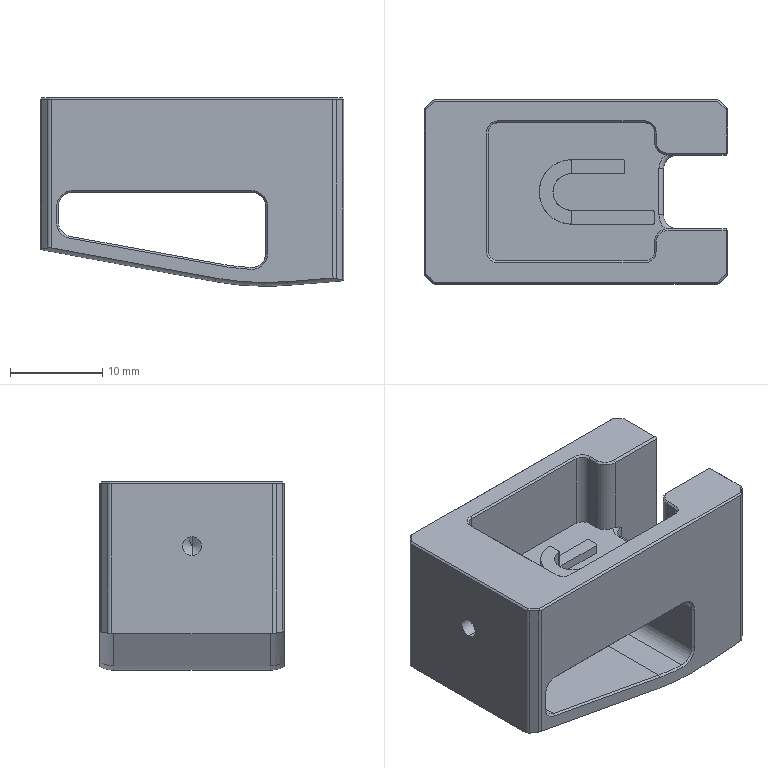Part | 1 solid | 134 faces | box 33 x 20 x 20.478 mm | volume 6105 mm3 | plane 66 | cylinder 40 | cone 20 | torus 4 | spline 4 | commonest cylinder face diameters 1 x9 3 x9 0.4 x8 2 x4 6 x4 2.05 x2